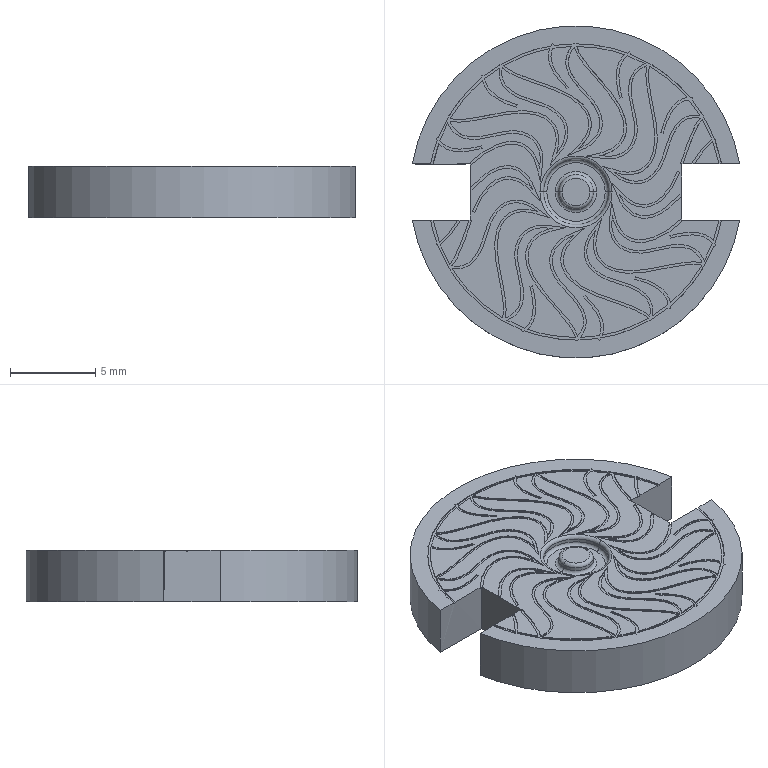Part | SolidWorks | features BaseBody 1 | 1 solid | 261 faces | box 19.154 x 19.434 x 3 mm | volume 813.614 mm3 | spline 180 | plane 67 | torus 8 | cylinder 6 | commonest cylinder face diameters 2.022 x2 3.822 x2 19.434 x2